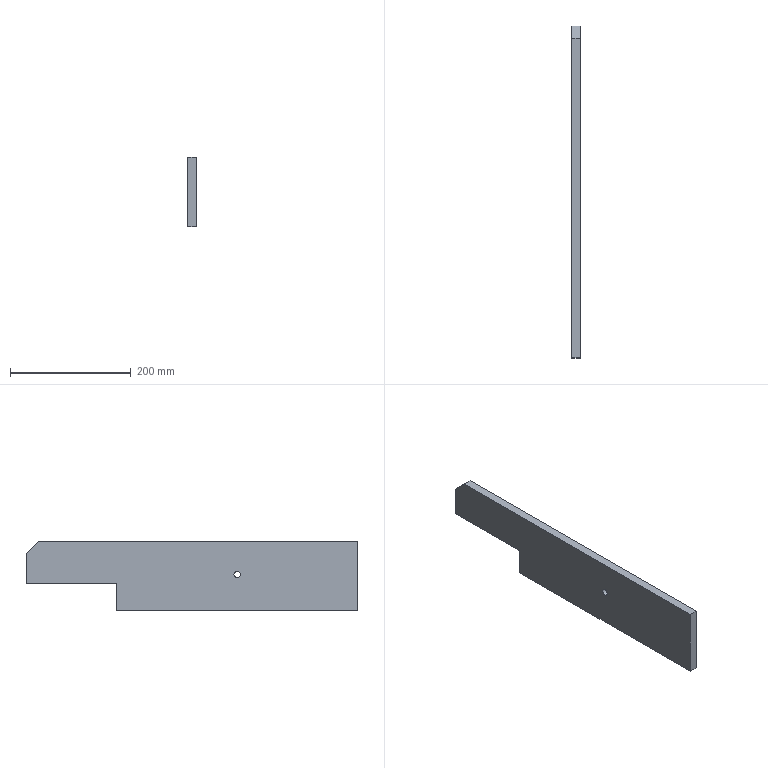Part | SolidWorks | features ICE 2, Chamfer 1, Extrusion 1 | 1 solid | 11 faces | box 14 x 550 x 115 mm | volume 786870 mm3 | plane 9 | cylinder 2 | commonest cylinder face diameters 11 x2
STEP:
#1=CARTESIAN_POINT('',(-7.,-200.,9.5));
#2=VERTEX_POINT('',#1);
#3=CARTESIAN_POINT('',(-7.,-200.,20.5));
#4=VERTEX_POINT('',#3);
#5=CARTESIAN_POINT('',(-7.,-200.,15.));
#6=DIRECTION('',(-1.,0.,0.));
#7=DIRECTION('',(0.,0.,-1.));
#8=AXIS2_PLACEMENT_3D('',#5,#6,#7);
#9=CIRCLE('',#8,5.5);
#10=EDGE_CURVE('',#2,#4,#9,.T.);
#11=ORIENTED_EDGE('',*,*,#10,.T.);
#12=CARTESIAN_POINT('',(7.,-200.,20.5));
#13=VERTEX_POINT('',#12);
#14=CARTESIAN_POINT('',(-7.001,-200.,20.5));
#15=DIRECTION('',(1.,0.,0.));
#16=VECTOR('',#15,1000.);
#17=LINE('',#14,#16);
#18=EDGE_CURVE('',#4,#13,#17,.T.);
#19=ORIENTED_EDGE('',*,*,#18,.T.);
#20=CARTESIAN_POINT('',(7.,-200.,9.5));
#21=VERTEX_POINT('',#20);
#22=CARTESIAN_POINT('',(7.,-200.,15.));
#23=DIRECTION('',(1.,0.,0.));
#24=DIRECTION('',(0.,0.,-1.));
#25=AXIS2_PLACEMENT_3D('',#22,#23,#24);
#26=CIRCLE('',#25,5.5);
#27=EDGE_CURVE('',#13,#21,#26,.T.);
#28=ORIENTED_EDGE('',*,*,#27,.T.);
#29=CARTESIAN_POINT('',(-7.001,-200.,9.5));
#30=DIRECTION('',(1.,0.,0.));
#31=VECTOR('',#30,1000.);
#32=LINE('',#29,#31);
#33=EDGE_CURVE('',#2,#21,#32,.T.);
#34=ORIENTED_EDGE('',*,*,#33,.F.);
#35=EDGE_LOOP('',(#11,#19,#28,#34));
#36=FACE_OUTER_BOUND('',#35,.T.);
#37=CARTESIAN_POINT('',(-7.001,-200.,15.));
#38=DIRECTION('',(1.,0.,0.));
#39=DIRECTION('',(0.,0.,-1.));
#40=AXIS2_PLACEMENT_3D('',#37,#38,#39);
#41=CYLINDRICAL_SURFACE('',#40,5.5);
#42=ADVANCED_FACE('',(#36),#41,.F.);
#43=CARTESIAN_POINT('',(-7.,0.,0.));
#44=VERTEX_POINT('',#43);
#45=CARTESIAN_POINT('',(-7.,150.,0.));
#46=VERTEX_POINT('',#45);
#47=CARTESIAN_POINT('',(-7.,150.,0.));
#48=DIRECTION('',(0.,1.,0.));
#49=VECTOR('',#48,1000.);
#50=LINE('',#47,#49);
#51=EDGE_CURVE('',#44,#46,#50,.T.);
#52=ORIENTED_EDGE('',*,*,#51,.T.);
#53=CARTESIAN_POINT('',(7.,150.,0.));
#54=VERTEX_POINT('',#53);
#55=CARTESIAN_POINT('',(7.,150.,0.));
#56=DIRECTION('',(-1.,0.,0.));
#57=VECTOR('',#56,1000.);
#58=LINE('',#55,#57);
#59=EDGE_CURVE('',#54,#46,#58,.T.);
#60=ORIENTED_EDGE('',*,*,#59,.F.);
#61=CARTESIAN_POINT('',(7.,0.,0.));
#62=VERTEX_POINT('',#61);
#63=CARTESIAN_POINT('',(7.,150.,0.));
#64=DIRECTION('',(0.,1.,0.));
#65=VECTOR('',#64,1000.);
#66=LINE('',#63,#65);
#67=EDGE_CURVE('',#62,#54,#66,.T.);
#68=ORIENTED_EDGE('',*,*,#67,.F.);
#69=CARTESIAN_POINT('',(7.,0.,0.));
#70=DIRECTION('',(-1.,0.,0.));
#71=VECTOR('',#70,1000.);
#72=LINE('',#69,#71);
#73=EDGE_CURVE('',#62,#44,#72,.T.);
#74=ORIENTED_EDGE('',*,*,#73,.T.);
#75=EDGE_LOOP('',(#52,#60,#68,#74));
#76=FACE_OUTER_BOUND('',#75,.T.);
#77=CARTESIAN_POINT('',(7.,150.,0.));
#78=DIRECTION('',(0.,0.,1.));
#79=DIRECTION('',(0.,-1.,0.));
#80=AXIS2_PLACEMENT_3D('',#77,#78,#79);
#81=PLANE('',#80);
#82=ADVANCED_FACE('',(#76),#81,.F.);
#83=CARTESIAN_POINT('',(-7.,150.,50.));
#84=VERTEX_POINT('',#83);
#85=CARTESIAN_POINT('',(-7.,150.,70.));
#86=DIRECTION('',(0.,0.,1.));
#87=VECTOR('',#86,1000.);
#88=LINE('',#85,#87);
#89=EDGE_CURVE('',#46,#84,#88,.T.);
#90=ORIENTED_EDGE('',*,*,#89,.T.);
#91=CARTESIAN_POINT('',(7.,150.,50.));
#92=VERTEX_POINT('',#91);
#93=CARTESIAN_POINT('',(7.,150.,50.));
#94=DIRECTION('',(1.,0.,0.));
#95=VECTOR('',#94,1000.);
#96=LINE('',#93,#95);
#97=EDGE_CURVE('',#84,#92,#96,.T.);
#98=ORIENTED_EDGE('',*,*,#97,.T.);
#99=CARTESIAN_POINT('',(7.,150.,70.));
#100=DIRECTION('',(0.,0.,1.));
#101=VECTOR('',#100,1000.);
#102=LINE('',#99,#101);
#103=EDGE_CURVE('',#54,#92,#102,.T.);
#104=ORIENTED_EDGE('',*,*,#103,.F.);
#105=ORIENTED_EDGE('',*,*,#59,.T.);
#106=EDGE_LOOP('',(#90,#98,#104,#105));
#107=FACE_OUTER_BOUND('',#106,.T.);
#108=CARTESIAN_POINT('',(7.,150.,70.));
#109=DIRECTION('',(0.,-1.,0.));
#110=DIRECTION('',(0.,0.,-1.));
#111=AXIS2_PLACEMENT_3D('',#108,#109,#110);
#112=PLANE('',#111);
#113=ADVANCED_FACE('',(#107),#112,.F.);
#114=CARTESIAN_POINT('',(7.,130.,70.));
#115=VERTEX_POINT('',#114);
#116=CARTESIAN_POINT('',(7.,-400.,70.));
#117=VERTEX_POINT('',#116);
#118=CARTESIAN_POINT('',(7.,-400.,70.));
#119=DIRECTION('',(0.,-1.,0.));
#120=VECTOR('',#119,1000.);
#121=LINE('',#118,#120);
#122=EDGE_CURVE('',#115,#117,#121,.T.);
#123=ORIENTED_EDGE('',*,*,#122,.F.);
#124=CARTESIAN_POINT('',(-7.,130.,70.));
#125=VERTEX_POINT('',#124);
#126=CARTESIAN_POINT('',(7.,130.,70.));
#127=DIRECTION('',(-1.,0.,0.));
#128=VECTOR('',#127,1000.);
#129=LINE('',#126,#128);
#130=EDGE_CURVE('',#115,#125,#129,.T.);
#131=ORIENTED_EDGE('',*,*,#130,.T.);
#132=CARTESIAN_POINT('',(-7.,-400.,70.));
#133=VERTEX_POINT('',#132);
#134=CARTESIAN_POINT('',(-7.,-400.,70.));
#135=DIRECTION('',(0.,-1.,0.));
#136=VECTOR('',#135,1000.);
#137=LINE('',#134,#136);
#138=EDGE_CURVE('',#125,#133,#137,.T.);
#139=ORIENTED_EDGE('',*,*,#138,.T.);
#140=CARTESIAN_POINT('',(7.,-400.,70.));
#141=DIRECTION('',(-1.,0.,0.));
#142=VECTOR('',#141,1000.);
#143=LINE('',#140,#142);
#144=EDGE_CURVE('',#117,#133,#143,.T.);
#145=ORIENTED_EDGE('',*,*,#144,.F.);
#146=EDGE_LOOP('',(#123,#131,#139,#145));
#147=FACE_OUTER_BOUND('',#146,.T.);
#148=CARTESIAN_POINT('',(7.,-400.,70.));
#149=DIRECTION('',(0.,0.,-1.));
#150=DIRECTION('',(-1.,0.,0.));
#151=AXIS2_PLACEMENT_3D('',#148,#149,#150);
#152=PLANE('',#151);
#153=ADVANCED_FACE('',(#147),#152,.F.);
#154=CARTESIAN_POINT('',(-7.,-400.,-45.));
#155=VERTEX_POINT('',#154);
#156=CARTESIAN_POINT('',(-7.,-400.,-45.));
#157=DIRECTION('',(0.,0.,-1.));
#158=VECTOR('',#157,1000.);
#159=LINE('',#156,#158);
#160=EDGE_CURVE('',#133,#155,#159,.T.);
#161=ORIENTED_EDGE('',*,*,#160,.T.);
#162=CARTESIAN_POINT('',(7.,-400.,-45.));
#163=VERTEX_POINT('',#162);
#164=CARTESIAN_POINT('',(7.,-400.,-45.));
#165=DIRECTION('',(-1.,0.,0.));
#166=VECTOR('',#165,1000.);
#167=LINE('',#164,#166);
#168=EDGE_CURVE('',#163,#155,#167,.T.);
#169=ORIENTED_EDGE('',*,*,#168,.F.);
#170=CARTESIAN_POINT('',(7.,-400.,-45.));
#171=DIRECTION('',(0.,0.,-1.));
#172=VECTOR('',#171,1000.);
#173=LINE('',#170,#172);
#174=EDGE_CURVE('',#117,#163,#173,.T.);
#175=ORIENTED_EDGE('',*,*,#174,.F.);
#176=ORIENTED_EDGE('',*,*,#144,.T.);
#177=EDGE_LOOP('',(#161,#169,#175,#176));
#178=FACE_OUTER_BOUND('',#177,.T.);
#179=CARTESIAN_POINT('',(7.,-400.,-45.));
#180=DIRECTION('',(0.,1.,0.));
#181=DIRECTION('',(0.,0.,1.));
#182=AXIS2_PLACEMENT_3D('',#179,#180,#181);
#183=PLANE('',#182);
#184=ADVANCED_FACE('',(#178),#183,.F.);
#185=CARTESIAN_POINT('',(-7.,0.,-45.));
#186=VERTEX_POINT('',#185);
#187=CARTESIAN_POINT('',(-7.,0.,-45.));
#188=DIRECTION('',(0.,1.,0.));
#189=VECTOR('',#188,1000.);
#190=LINE('',#187,#189);
#191=EDGE_CURVE('',#155,#186,#190,.T.);
#192=ORIENTED_EDGE('',*,*,#191,.T.);
#193=CARTESIAN_POINT('',(7.,0.,-45.));
#194=VERTEX_POINT('',#193);
#195=CARTESIAN_POINT('',(7.,0.,-45.));
#196=DIRECTION('',(-1.,0.,0.));
#197=VECTOR('',#196,1000.);
#198=LINE('',#195,#197);
#199=EDGE_CURVE('',#194,#186,#198,.T.);
#200=ORIENTED_EDGE('',*,*,#199,.F.);
#201=CARTESIAN_POINT('',(7.,0.,-45.));
#202=DIRECTION('',(0.,1.,0.));
#203=VECTOR('',#202,1000.);
#204=LINE('',#201,#203);
#205=EDGE_CURVE('',#163,#194,#204,.T.);
#206=ORIENTED_EDGE('',*,*,#205,.F.);
#207=ORIENTED_EDGE('',*,*,#168,.T.);
#208=EDGE_LOOP('',(#192,#200,#206,#207));
#209=FACE_OUTER_BOUND('',#208,.T.);
#210=CARTESIAN_POINT('',(7.,0.,-45.));
#211=DIRECTION('',(0.,0.,1.));
#212=DIRECTION('',(0.,-1.,0.));
#213=AXIS2_PLACEMENT_3D('',#210,#211,#212);
#214=PLANE('',#213);
#215=ADVANCED_FACE('',(#209),#214,.F.);
#216=CARTESIAN_POINT('',(-7.,0.,0.));
#217=DIRECTION('',(0.,0.,1.));
#218=VECTOR('',#217,1000.);
#219=LINE('',#216,#218);
#220=EDGE_CURVE('',#186,#44,#219,.T.);
#221=ORIENTED_EDGE('',*,*,#220,.T.);
#222=ORIENTED_EDGE('',*,*,#73,.F.);
#223=CARTESIAN_POINT('',(7.,0.,0.));
#224=DIRECTION('',(0.,0.,1.));
#225=VECTOR('',#224,1000.);
#226=LINE('',#223,#225);
#227=EDGE_CURVE('',#194,#62,#226,.T.);
#228=ORIENTED_EDGE('',*,*,#227,.F.);
#229=ORIENTED_EDGE('',*,*,#199,.T.);
#230=EDGE_LOOP('',(#221,#222,#228,#229));
#231=FACE_OUTER_BOUND('',#230,.T.);
#232=CARTESIAN_POINT('',(7.,0.,0.));
#233=DIRECTION('',(0.,-1.,0.));
#234=DIRECTION('',(0.,0.,-1.));
#235=AXIS2_PLACEMENT_3D('',#232,#233,#234);
#236=PLANE('',#235);
#237=ADVANCED_FACE('',(#231),#236,.F.);
#238=CARTESIAN_POINT('',(7.,-200.,15.));
#239=DIRECTION('',(1.,0.,0.));
#240=DIRECTION('',(0.,0.,-1.));
#241=AXIS2_PLACEMENT_3D('',#238,#239,#240);
#242=CIRCLE('',#241,5.5);
#243=EDGE_CURVE('',#21,#13,#242,.T.);
#244=ORIENTED_EDGE('',*,*,#243,.F.);
#245=ORIENTED_EDGE('',*,*,#27,.F.);
#246=EDGE_LOOP('',(#244,#245));
#247=FACE_BOUND('',#246,.T.);
#248=ORIENTED_EDGE('',*,*,#103,.T.);
#249=CARTESIAN_POINT('',(7.,100.,100.));
#250=DIRECTION('',(0.,-0.7071,0.7071));
#251=VECTOR('',#250,1000.);
#252=LINE('',#249,#251);
#253=EDGE_CURVE('',#92,#115,#252,.T.);
#254=ORIENTED_EDGE('',*,*,#253,.T.);
#255=ORIENTED_EDGE('',*,*,#122,.T.);
#256=ORIENTED_EDGE('',*,*,#174,.T.);
#257=ORIENTED_EDGE('',*,*,#205,.T.);
#258=ORIENTED_EDGE('',*,*,#227,.T.);
#259=ORIENTED_EDGE('',*,*,#67,.T.);
#260=EDGE_LOOP('',(#248,#254,#255,#256,#257,#258,#259));
#261=FACE_OUTER_BOUND('',#260,.T.);
#262=CARTESIAN_POINT('',(7.,0.,0.));
#263=DIRECTION('',(1.,0.,0.));
#264=DIRECTION('',(0.,0.,-1.));
#265=AXIS2_PLACEMENT_3D('',#262,#263,#264);
#266=PLANE('',#265);
#267=ADVANCED_FACE('',(#247,#261),#266,.T.);
#268=ORIENTED_EDGE('',*,*,#10,.F.);
#269=CARTESIAN_POINT('',(-7.,-200.,15.));
#270=DIRECTION('',(-1.,0.,0.));
#271=DIRECTION('',(0.,0.,-1.));
#272=AXIS2_PLACEMENT_3D('',#269,#270,#271);
#273=CIRCLE('',#272,5.5);
#274=EDGE_CURVE('',#4,#2,#273,.T.);
#275=ORIENTED_EDGE('',*,*,#274,.F.);
#276=EDGE_LOOP('',(#268,#275));
#277=FACE_BOUND('',#276,.T.);
#278=ORIENTED_EDGE('',*,*,#138,.F.);
#279=CARTESIAN_POINT('',(-7.,130.,70.));
#280=DIRECTION('',(0.,0.7071,-0.7071));
#281=VECTOR('',#280,1000.);
#282=LINE('',#279,#281);
#283=EDGE_CURVE('',#125,#84,#282,.T.);
#284=ORIENTED_EDGE('',*,*,#283,.T.);
#285=ORIENTED_EDGE('',*,*,#89,.F.);
#286=ORIENTED_EDGE('',*,*,#51,.F.);
#287=ORIENTED_EDGE('',*,*,#220,.F.);
#288=ORIENTED_EDGE('',*,*,#191,.F.);
#289=ORIENTED_EDGE('',*,*,#160,.F.);
#290=EDGE_LOOP('',(#278,#284,#285,#286,#287,#288,#289));
#291=FACE_OUTER_BOUND('',#290,.T.);
#292=CARTESIAN_POINT('',(-7.,0.,0.));
#293=DIRECTION('',(1.,0.,0.));
#294=DIRECTION('',(0.,0.,-1.));
#295=AXIS2_PLACEMENT_3D('',#292,#293,#294);
#296=PLANE('',#295);
#297=ADVANCED_FACE('',(#277,#291),#296,.F.);
#298=ORIENTED_EDGE('',*,*,#18,.F.);
#299=ORIENTED_EDGE('',*,*,#274,.T.);
#300=ORIENTED_EDGE('',*,*,#33,.T.);
#301=ORIENTED_EDGE('',*,*,#243,.T.);
#302=EDGE_LOOP('',(#298,#299,#300,#301));
#303=FACE_OUTER_BOUND('',#302,.T.);
#304=CARTESIAN_POINT('',(-7.001,-200.,15.));
#305=DIRECTION('',(1.,0.,0.));
#306=DIRECTION('',(0.,0.,-1.));
#307=AXIS2_PLACEMENT_3D('',#304,#305,#306);
#308=CYLINDRICAL_SURFACE('',#307,5.5);
#309=ADVANCED_FACE('',(#303),#308,.F.);
#310=ORIENTED_EDGE('',*,*,#253,.F.);
#311=ORIENTED_EDGE('',*,*,#97,.F.);
#312=ORIENTED_EDGE('',*,*,#283,.F.);
#313=ORIENTED_EDGE('',*,*,#130,.F.);
#314=EDGE_LOOP('',(#310,#311,#312,#313));
#315=FACE_OUTER_BOUND('',#314,.T.);
#316=CARTESIAN_POINT('',(7.,130.,70.));
#317=DIRECTION('',(0.,-0.7071,-0.7071));
#318=DIRECTION('',(-1.,0.,0.));
#319=AXIS2_PLACEMENT_3D('',#316,#317,#318);
#320=PLANE('',#319);
#321=ADVANCED_FACE('',(#315),#320,.F.);
#322=CLOSED_SHELL('',(#42,#82,#113,#153,#184,#215,#237,#267,#297,#309,#321));
#323=MANIFOLD_SOLID_BREP('',#322);
#324=CARTESIAN_POINT('',(0.,0.,0.));
#325=DIRECTION('',(0.,0.,1.));
#326=DIRECTION('',(1.,0.,0.));
#327=AXIS2_PLACEMENT_3D('',#324,#325,#326);
#328=(LENGTH_UNIT()NAMED_UNIT(*)SI_UNIT(.MILLI.,.METRE.));
#329=UNCERTAINTY_MEASURE_WITH_UNIT(LENGTH_MEASURE(0.00001),#328,'','');
#330=(NAMED_UNIT(*)PLANE_ANGLE_UNIT()SI_UNIT($,.RADIAN.));
#331=(NAMED_UNIT(*)SI_UNIT($,.STERADIAN.)SOLID_ANGLE_UNIT());
#332=(GEOMETRIC_REPRESENTATION_CONTEXT(3)GLOBAL_UNCERTAINTY_ASSIGNED_CONTEXT((#329))GLOBAL_UNIT_ASSIGNED_CONTEXT((#328,#330,#331))REPRESENTATION_CONTEXT('',''));
#333=ADVANCED_BREP_SHAPE_REPRESENTATION('',(#323,#327),#332);